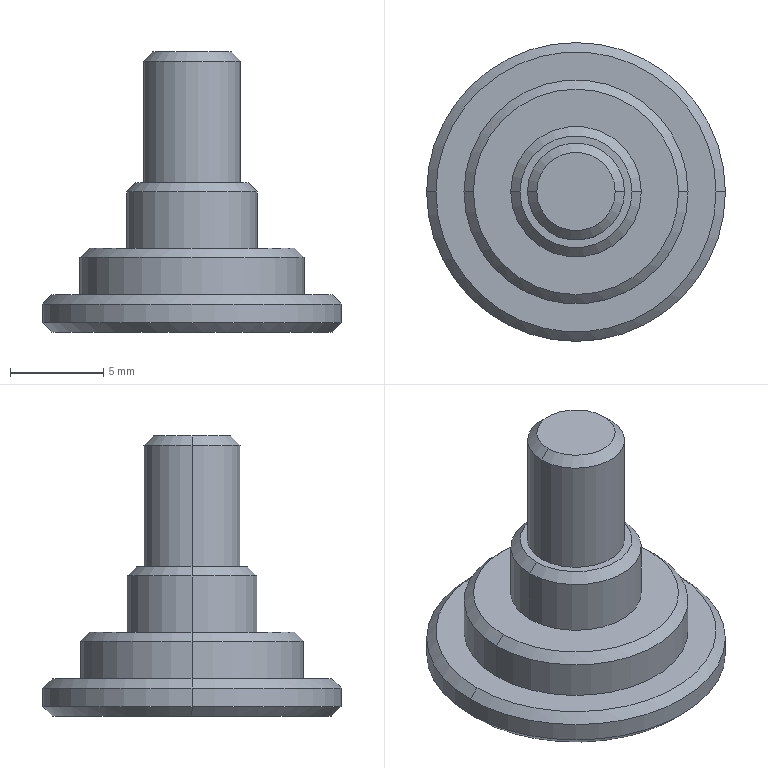Part | SolidWorks | features Boss 3, Chamfer 1, FlatPattern 1, SMBaseFlange 1, SheetMetal 1 | 1 solid | 23 faces | box 16 x 16 x 15 mm | volume 946.808 mm3 | cone 10 | cylinder 8 | plane 5 | commonest cylinder face diameters 5.2 x2 7 x2 12 x2 16 x2
STEP:
#1=CARTESIAN_POINT('',(2.1,0.,15.));
#2=VERTEX_POINT('',#1);
#3=CARTESIAN_POINT('',(-2.1,0.,15.));
#4=VERTEX_POINT('',#3);
#5=CARTESIAN_POINT('',(0.,0.,15.));
#6=DIRECTION('',(0.,0.,1.));
#7=DIRECTION('',(1.,0.,0.));
#8=AXIS2_PLACEMENT_3D('',#5,#6,#7);
#9=CIRCLE('',#8,2.1);
#10=EDGE_CURVE('',#2,#4,#9,.T.);
#11=ORIENTED_EDGE('',*,*,#10,.F.);
#12=CARTESIAN_POINT('',(2.6,0.,14.5));
#13=VERTEX_POINT('',#12);
#14=CARTESIAN_POINT('',(2.1,0.,15.));
#15=DIRECTION('',(0.7071,0.,-0.7071));
#16=VECTOR('',#15,1000.);
#17=LINE('',#14,#16);
#18=EDGE_CURVE('',#2,#13,#17,.T.);
#19=ORIENTED_EDGE('',*,*,#18,.T.);
#20=CARTESIAN_POINT('',(-2.6,0.,14.5));
#21=VERTEX_POINT('',#20);
#22=CARTESIAN_POINT('',(0.,0.,14.5));
#23=DIRECTION('',(0.,0.,-1.));
#24=DIRECTION('',(1.,0.,0.));
#25=AXIS2_PLACEMENT_3D('',#22,#23,#24);
#26=CIRCLE('',#25,2.6);
#27=EDGE_CURVE('',#21,#13,#26,.T.);
#28=ORIENTED_EDGE('',*,*,#27,.F.);
#29=CARTESIAN_POINT('',(-2.1,0.,15.));
#30=DIRECTION('',(-0.7071,0.,-0.7071));
#31=VECTOR('',#30,1000.);
#32=LINE('',#29,#31);
#33=EDGE_CURVE('',#4,#21,#32,.T.);
#34=ORIENTED_EDGE('',*,*,#33,.F.);
#35=EDGE_LOOP('',(#11,#19,#28,#34));
#36=FACE_OUTER_BOUND('',#35,.T.);
#37=CARTESIAN_POINT('',(0.,0.,15.));
#38=DIRECTION('',(0.,0.,-1.));
#39=DIRECTION('',(-1.,0.,0.));
#40=AXIS2_PLACEMENT_3D('',#37,#38,#39);
#41=CONICAL_SURFACE('',#40,2.1,0.7854);
#42=ADVANCED_FACE('',(#36),#41,.T.);
#43=CARTESIAN_POINT('',(3.,0.,8.));
#44=VERTEX_POINT('',#43);
#45=CARTESIAN_POINT('',(-3.,0.,8.));
#46=VERTEX_POINT('',#45);
#47=CARTESIAN_POINT('',(0.,0.,8.));
#48=DIRECTION('',(0.,0.,1.));
#49=DIRECTION('',(1.,0.,0.));
#50=AXIS2_PLACEMENT_3D('',#47,#48,#49);
#51=CIRCLE('',#50,3.);
#52=EDGE_CURVE('',#44,#46,#51,.T.);
#53=ORIENTED_EDGE('',*,*,#52,.F.);
#54=CARTESIAN_POINT('',(3.5,0.,7.5));
#55=VERTEX_POINT('',#54);
#56=CARTESIAN_POINT('',(3.,0.,8.));
#57=DIRECTION('',(0.7071,0.,-0.7071));
#58=VECTOR('',#57,1000.);
#59=LINE('',#56,#58);
#60=EDGE_CURVE('',#44,#55,#59,.T.);
#61=ORIENTED_EDGE('',*,*,#60,.T.);
#62=CARTESIAN_POINT('',(-3.5,0.,7.5));
#63=VERTEX_POINT('',#62);
#64=CARTESIAN_POINT('',(0.,0.,7.5));
#65=DIRECTION('',(0.,0.,-1.));
#66=DIRECTION('',(1.,0.,0.));
#67=AXIS2_PLACEMENT_3D('',#64,#65,#66);
#68=CIRCLE('',#67,3.5);
#69=EDGE_CURVE('',#63,#55,#68,.T.);
#70=ORIENTED_EDGE('',*,*,#69,.F.);
#71=CARTESIAN_POINT('',(-3.,0.,8.));
#72=DIRECTION('',(-0.7071,0.,-0.7071));
#73=VECTOR('',#72,1000.);
#74=LINE('',#71,#73);
#75=EDGE_CURVE('',#46,#63,#74,.T.);
#76=ORIENTED_EDGE('',*,*,#75,.F.);
#77=EDGE_LOOP('',(#53,#61,#70,#76));
#78=FACE_OUTER_BOUND('',#77,.T.);
#79=CARTESIAN_POINT('',(0.,0.,8.));
#80=DIRECTION('',(0.,0.,-1.));
#81=DIRECTION('',(-1.,0.,0.));
#82=AXIS2_PLACEMENT_3D('',#79,#80,#81);
#83=CONICAL_SURFACE('',#82,3.,0.7854);
#84=ADVANCED_FACE('',(#78),#83,.T.);
#85=CARTESIAN_POINT('',(5.5,0.,4.5));
#86=VERTEX_POINT('',#85);
#87=CARTESIAN_POINT('',(-5.5,0.,4.5));
#88=VERTEX_POINT('',#87);
#89=CARTESIAN_POINT('',(0.,0.,4.5));
#90=DIRECTION('',(0.,0.,1.));
#91=DIRECTION('',(1.,0.,0.));
#92=AXIS2_PLACEMENT_3D('',#89,#90,#91);
#93=CIRCLE('',#92,5.5);
#94=EDGE_CURVE('',#86,#88,#93,.T.);
#95=ORIENTED_EDGE('',*,*,#94,.F.);
#96=CARTESIAN_POINT('',(6.,0.,4.));
#97=VERTEX_POINT('',#96);
#98=CARTESIAN_POINT('',(5.5,0.,4.5));
#99=DIRECTION('',(0.7071,0.,-0.7071));
#100=VECTOR('',#99,1000.);
#101=LINE('',#98,#100);
#102=EDGE_CURVE('',#86,#97,#101,.T.);
#103=ORIENTED_EDGE('',*,*,#102,.T.);
#104=CARTESIAN_POINT('',(-6.,0.,4.));
#105=VERTEX_POINT('',#104);
#106=CARTESIAN_POINT('',(0.,0.,4.));
#107=DIRECTION('',(0.,0.,-1.));
#108=DIRECTION('',(1.,0.,0.));
#109=AXIS2_PLACEMENT_3D('',#106,#107,#108);
#110=CIRCLE('',#109,6.);
#111=EDGE_CURVE('',#105,#97,#110,.T.);
#112=ORIENTED_EDGE('',*,*,#111,.F.);
#113=CARTESIAN_POINT('',(-5.5,0.,4.5));
#114=DIRECTION('',(-0.7071,0.,-0.7071));
#115=VECTOR('',#114,1000.);
#116=LINE('',#113,#115);
#117=EDGE_CURVE('',#88,#105,#116,.T.);
#118=ORIENTED_EDGE('',*,*,#117,.F.);
#119=EDGE_LOOP('',(#95,#103,#112,#118));
#120=FACE_OUTER_BOUND('',#119,.T.);
#121=CARTESIAN_POINT('',(0.,0.,4.5));
#122=DIRECTION('',(0.,0.,-1.));
#123=DIRECTION('',(-1.,0.,0.));
#124=AXIS2_PLACEMENT_3D('',#121,#122,#123);
#125=CONICAL_SURFACE('',#124,5.5,0.7854);
#126=ADVANCED_FACE('',(#120),#125,.T.);
#127=CARTESIAN_POINT('',(7.5,0.,2.));
#128=VERTEX_POINT('',#127);
#129=CARTESIAN_POINT('',(-7.5,0.,2.));
#130=VERTEX_POINT('',#129);
#131=CARTESIAN_POINT('',(0.,0.,2.));
#132=DIRECTION('',(0.,0.,1.));
#133=DIRECTION('',(1.,0.,0.));
#134=AXIS2_PLACEMENT_3D('',#131,#132,#133);
#135=CIRCLE('',#134,7.5);
#136=EDGE_CURVE('',#128,#130,#135,.T.);
#137=ORIENTED_EDGE('',*,*,#136,.F.);
#138=CARTESIAN_POINT('',(8.,0.,1.5));
#139=VERTEX_POINT('',#138);
#140=CARTESIAN_POINT('',(7.5,0.,2.));
#141=DIRECTION('',(0.7071,0.,-0.7071));
#142=VECTOR('',#141,1000.);
#143=LINE('',#140,#142);
#144=EDGE_CURVE('',#128,#139,#143,.T.);
#145=ORIENTED_EDGE('',*,*,#144,.T.);
#146=CARTESIAN_POINT('',(-8.,0.,1.5));
#147=VERTEX_POINT('',#146);
#148=CARTESIAN_POINT('',(0.,0.,1.5));
#149=DIRECTION('',(0.,0.,-1.));
#150=DIRECTION('',(1.,0.,0.));
#151=AXIS2_PLACEMENT_3D('',#148,#149,#150);
#152=CIRCLE('',#151,8.);
#153=EDGE_CURVE('',#147,#139,#152,.T.);
#154=ORIENTED_EDGE('',*,*,#153,.F.);
#155=CARTESIAN_POINT('',(-7.5,0.,2.));
#156=DIRECTION('',(-0.7071,0.,-0.7071));
#157=VECTOR('',#156,1000.);
#158=LINE('',#155,#157);
#159=EDGE_CURVE('',#130,#147,#158,.T.);
#160=ORIENTED_EDGE('',*,*,#159,.F.);
#161=EDGE_LOOP('',(#137,#145,#154,#160));
#162=FACE_OUTER_BOUND('',#161,.T.);
#163=CARTESIAN_POINT('',(0.,0.,2.));
#164=DIRECTION('',(0.,0.,-1.));
#165=DIRECTION('',(-1.,0.,0.));
#166=AXIS2_PLACEMENT_3D('',#163,#164,#165);
#167=CONICAL_SURFACE('',#166,7.5,0.7854);
#168=ADVANCED_FACE('',(#162),#167,.T.);
#169=CARTESIAN_POINT('',(-7.5,0.,0.));
#170=VERTEX_POINT('',#169);
#171=CARTESIAN_POINT('',(7.5,0.,0.));
#172=VERTEX_POINT('',#171);
#173=CARTESIAN_POINT('',(0.,0.,0.));
#174=DIRECTION('',(0.,0.,-1.));
#175=DIRECTION('',(1.,0.,0.));
#176=AXIS2_PLACEMENT_3D('',#173,#174,#175);
#177=CIRCLE('',#176,7.5);
#178=EDGE_CURVE('',#170,#172,#177,.T.);
#179=ORIENTED_EDGE('',*,*,#178,.F.);
#180=CARTESIAN_POINT('',(-8.,0.,0.5));
#181=VERTEX_POINT('',#180);
#182=CARTESIAN_POINT('',(-8.,0.,0.5));
#183=DIRECTION('',(-0.7071,0.,0.7071));
#184=VECTOR('',#183,1000.);
#185=LINE('',#182,#184);
#186=EDGE_CURVE('',#170,#181,#185,.T.);
#187=ORIENTED_EDGE('',*,*,#186,.T.);
#188=CARTESIAN_POINT('',(8.,0.,0.5));
#189=VERTEX_POINT('',#188);
#190=CARTESIAN_POINT('',(0.,0.,0.5));
#191=DIRECTION('',(0.,0.,1.));
#192=DIRECTION('',(1.,0.,0.));
#193=AXIS2_PLACEMENT_3D('',#190,#191,#192);
#194=CIRCLE('',#193,8.);
#195=EDGE_CURVE('',#189,#181,#194,.T.);
#196=ORIENTED_EDGE('',*,*,#195,.F.);
#197=CARTESIAN_POINT('',(8.,0.,0.5));
#198=DIRECTION('',(0.7071,0.,0.7071));
#199=VECTOR('',#198,1000.);
#200=LINE('',#197,#199);
#201=EDGE_CURVE('',#172,#189,#200,.T.);
#202=ORIENTED_EDGE('',*,*,#201,.F.);
#203=EDGE_LOOP('',(#179,#187,#196,#202));
#204=FACE_OUTER_BOUND('',#203,.T.);
#205=CARTESIAN_POINT('',(0.,0.,0.5));
#206=DIRECTION('',(0.,0.,1.));
#207=DIRECTION('',(1.,0.,0.));
#208=AXIS2_PLACEMENT_3D('',#205,#206,#207);
#209=CONICAL_SURFACE('',#208,8.,0.7854);
#210=ADVANCED_FACE('',(#204),#209,.T.);
#211=ORIENTED_EDGE('',*,*,#27,.T.);
#212=CARTESIAN_POINT('',(2.6,0.,8.));
#213=VERTEX_POINT('',#212);
#214=CARTESIAN_POINT('',(2.6,0.,15.));
#215=DIRECTION('',(0.,0.,-1.));
#216=VECTOR('',#215,1000.);
#217=LINE('',#214,#216);
#218=EDGE_CURVE('',#13,#213,#217,.T.);
#219=ORIENTED_EDGE('',*,*,#218,.T.);
#220=CARTESIAN_POINT('',(-2.6,0.,8.));
#221=VERTEX_POINT('',#220);
#222=CARTESIAN_POINT('',(0.,0.,8.));
#223=DIRECTION('',(0.,0.,1.));
#224=DIRECTION('',(1.,0.,0.));
#225=AXIS2_PLACEMENT_3D('',#222,#223,#224);
#226=CIRCLE('',#225,2.6);
#227=EDGE_CURVE('',#213,#221,#226,.T.);
#228=ORIENTED_EDGE('',*,*,#227,.T.);
#229=CARTESIAN_POINT('',(-2.6,0.,15.));
#230=DIRECTION('',(0.,0.,-1.));
#231=VECTOR('',#230,1000.);
#232=LINE('',#229,#231);
#233=EDGE_CURVE('',#21,#221,#232,.T.);
#234=ORIENTED_EDGE('',*,*,#233,.F.);
#235=EDGE_LOOP('',(#211,#219,#228,#234));
#236=FACE_OUTER_BOUND('',#235,.T.);
#237=CARTESIAN_POINT('',(0.,0.,15.));
#238=DIRECTION('',(0.,0.,-1.));
#239=DIRECTION('',(-1.,0.,0.));
#240=AXIS2_PLACEMENT_3D('',#237,#238,#239);
#241=CYLINDRICAL_SURFACE('',#240,2.6);
#242=ADVANCED_FACE('',(#236),#241,.T.);
#243=ORIENTED_EDGE('',*,*,#69,.T.);
#244=CARTESIAN_POINT('',(3.5,0.,4.5));
#245=VERTEX_POINT('',#244);
#246=CARTESIAN_POINT('',(3.5,0.,8.));
#247=DIRECTION('',(0.,0.,-1.));
#248=VECTOR('',#247,1000.);
#249=LINE('',#246,#248);
#250=EDGE_CURVE('',#55,#245,#249,.T.);
#251=ORIENTED_EDGE('',*,*,#250,.T.);
#252=CARTESIAN_POINT('',(-3.5,0.,4.5));
#253=VERTEX_POINT('',#252);
#254=CARTESIAN_POINT('',(0.,0.,4.5));
#255=DIRECTION('',(0.,0.,1.));
#256=DIRECTION('',(1.,0.,0.));
#257=AXIS2_PLACEMENT_3D('',#254,#255,#256);
#258=CIRCLE('',#257,3.5);
#259=EDGE_CURVE('',#245,#253,#258,.T.);
#260=ORIENTED_EDGE('',*,*,#259,.T.);
#261=CARTESIAN_POINT('',(-3.5,0.,8.));
#262=DIRECTION('',(0.,0.,-1.));
#263=VECTOR('',#262,1000.);
#264=LINE('',#261,#263);
#265=EDGE_CURVE('',#63,#253,#264,.T.);
#266=ORIENTED_EDGE('',*,*,#265,.F.);
#267=EDGE_LOOP('',(#243,#251,#260,#266));
#268=FACE_OUTER_BOUND('',#267,.T.);
#269=CARTESIAN_POINT('',(0.,0.,8.));
#270=DIRECTION('',(0.,0.,-1.));
#271=DIRECTION('',(-1.,0.,0.));
#272=AXIS2_PLACEMENT_3D('',#269,#270,#271);
#273=CYLINDRICAL_SURFACE('',#272,3.5);
#274=ADVANCED_FACE('',(#268),#273,.T.);
#275=ORIENTED_EDGE('',*,*,#111,.T.);
#276=CARTESIAN_POINT('',(6.,0.,2.));
#277=VERTEX_POINT('',#276);
#278=CARTESIAN_POINT('',(6.,0.,4.5));
#279=DIRECTION('',(0.,0.,-1.));
#280=VECTOR('',#279,1000.);
#281=LINE('',#278,#280);
#282=EDGE_CURVE('',#97,#277,#281,.T.);
#283=ORIENTED_EDGE('',*,*,#282,.T.);
#284=CARTESIAN_POINT('',(-6.,0.,2.));
#285=VERTEX_POINT('',#284);
#286=CARTESIAN_POINT('',(0.,0.,2.));
#287=DIRECTION('',(0.,0.,1.));
#288=DIRECTION('',(1.,0.,0.));
#289=AXIS2_PLACEMENT_3D('',#286,#287,#288);
#290=CIRCLE('',#289,6.);
#291=EDGE_CURVE('',#277,#285,#290,.T.);
#292=ORIENTED_EDGE('',*,*,#291,.T.);
#293=CARTESIAN_POINT('',(-6.,0.,4.5));
#294=DIRECTION('',(0.,0.,-1.));
#295=VECTOR('',#294,1000.);
#296=LINE('',#293,#295);
#297=EDGE_CURVE('',#105,#285,#296,.T.);
#298=ORIENTED_EDGE('',*,*,#297,.F.);
#299=EDGE_LOOP('',(#275,#283,#292,#298));
#300=FACE_OUTER_BOUND('',#299,.T.);
#301=CARTESIAN_POINT('',(0.,0.,4.5));
#302=DIRECTION('',(0.,0.,-1.));
#303=DIRECTION('',(-1.,0.,0.));
#304=AXIS2_PLACEMENT_3D('',#301,#302,#303);
#305=CYLINDRICAL_SURFACE('',#304,6.);
#306=ADVANCED_FACE('',(#300),#305,.T.);
#307=ORIENTED_EDGE('',*,*,#153,.T.);
#308=CARTESIAN_POINT('',(8.,0.,2.));
#309=DIRECTION('',(0.,0.,-1.));
#310=VECTOR('',#309,1000.);
#311=LINE('',#308,#310);
#312=EDGE_CURVE('',#139,#189,#311,.T.);
#313=ORIENTED_EDGE('',*,*,#312,.T.);
#314=ORIENTED_EDGE('',*,*,#195,.T.);
#315=CARTESIAN_POINT('',(-8.,0.,2.));
#316=DIRECTION('',(0.,0.,-1.));
#317=VECTOR('',#316,1000.);
#318=LINE('',#315,#317);
#319=EDGE_CURVE('',#147,#181,#318,.T.);
#320=ORIENTED_EDGE('',*,*,#319,.F.);
#321=EDGE_LOOP('',(#307,#313,#314,#320));
#322=FACE_OUTER_BOUND('',#321,.T.);
#323=CARTESIAN_POINT('',(0.,0.,2.));
#324=DIRECTION('',(0.,0.,-1.));
#325=DIRECTION('',(-1.,0.,0.));
#326=AXIS2_PLACEMENT_3D('',#323,#324,#325);
#327=CYLINDRICAL_SURFACE('',#326,8.);
#328=ADVANCED_FACE('',(#322),#327,.T.);
#329=CARTESIAN_POINT('',(0.,0.,8.));
#330=DIRECTION('',(0.,0.,1.));
#331=DIRECTION('',(1.,0.,0.));
#332=AXIS2_PLACEMENT_3D('',#329,#330,#331);
#333=CIRCLE('',#332,3.);
#334=EDGE_CURVE('',#46,#44,#333,.T.);
#335=ORIENTED_EDGE('',*,*,#334,.T.);
#336=ORIENTED_EDGE('',*,*,#52,.T.);
#337=EDGE_LOOP('',(#335,#336));
#338=FACE_OUTER_BOUND('',#337,.T.);
#339=CARTESIAN_POINT('',(0.,0.,8.));
#340=DIRECTION('',(0.,0.,1.));
#341=DIRECTION('',(1.,0.,0.));
#342=AXIS2_PLACEMENT_3D('',#339,#340,#341);
#343=CIRCLE('',#342,2.6);
#344=EDGE_CURVE('',#221,#213,#343,.T.);
#345=ORIENTED_EDGE('',*,*,#344,.F.);
#346=ORIENTED_EDGE('',*,*,#227,.F.);
#347=EDGE_LOOP('',(#345,#346));
#348=FACE_BOUND('',#347,.T.);
#349=CARTESIAN_POINT('',(0.,0.,8.));
#350=DIRECTION('',(0.,0.,1.));
#351=DIRECTION('',(1.,0.,0.));
#352=AXIS2_PLACEMENT_3D('',#349,#350,#351);
#353=PLANE('',#352);
#354=ADVANCED_FACE('',(#338,#348),#353,.T.);
#355=CARTESIAN_POINT('',(0.,0.,4.5));
#356=DIRECTION('',(0.,0.,1.));
#357=DIRECTION('',(1.,0.,0.));
#358=AXIS2_PLACEMENT_3D('',#355,#356,#357);
#359=CIRCLE('',#358,5.5);
#360=EDGE_CURVE('',#88,#86,#359,.T.);
#361=ORIENTED_EDGE('',*,*,#360,.T.);
#362=ORIENTED_EDGE('',*,*,#94,.T.);
#363=EDGE_LOOP('',(#361,#362));
#364=FACE_OUTER_BOUND('',#363,.T.);
#365=CARTESIAN_POINT('',(0.,0.,4.5));
#366=DIRECTION('',(0.,0.,1.));
#367=DIRECTION('',(1.,0.,0.));
#368=AXIS2_PLACEMENT_3D('',#365,#366,#367);
#369=CIRCLE('',#368,3.5);
#370=EDGE_CURVE('',#253,#245,#369,.T.);
#371=ORIENTED_EDGE('',*,*,#370,.F.);
#372=ORIENTED_EDGE('',*,*,#259,.F.);
#373=EDGE_LOOP('',(#371,#372));
#374=FACE_BOUND('',#373,.T.);
#375=CARTESIAN_POINT('',(0.,0.,4.5));
#376=DIRECTION('',(0.,0.,1.));
#377=DIRECTION('',(1.,0.,0.));
#378=AXIS2_PLACEMENT_3D('',#375,#376,#377);
#379=PLANE('',#378);
#380=ADVANCED_FACE('',(#364,#374),#379,.T.);
#381=CARTESIAN_POINT('',(0.,0.,2.));
#382=DIRECTION('',(0.,0.,1.));
#383=DIRECTION('',(1.,0.,0.));
#384=AXIS2_PLACEMENT_3D('',#381,#382,#383);
#385=CIRCLE('',#384,7.5);
#386=EDGE_CURVE('',#130,#128,#385,.T.);
#387=ORIENTED_EDGE('',*,*,#386,.T.);
#388=ORIENTED_EDGE('',*,*,#136,.T.);
#389=EDGE_LOOP('',(#387,#388));
#390=FACE_OUTER_BOUND('',#389,.T.);
#391=CARTESIAN_POINT('',(0.,0.,2.));
#392=DIRECTION('',(0.,0.,1.));
#393=DIRECTION('',(1.,0.,0.));
#394=AXIS2_PLACEMENT_3D('',#391,#392,#393);
#395=CIRCLE('',#394,6.);
#396=EDGE_CURVE('',#285,#277,#395,.T.);
#397=ORIENTED_EDGE('',*,*,#396,.F.);
#398=ORIENTED_EDGE('',*,*,#291,.F.);
#399=EDGE_LOOP('',(#397,#398));
#400=FACE_BOUND('',#399,.T.);
#401=CARTESIAN_POINT('',(0.,0.,2.));
#402=DIRECTION('',(0.,0.,1.));
#403=DIRECTION('',(1.,0.,0.));
#404=AXIS2_PLACEMENT_3D('',#401,#402,#403);
#405=PLANE('',#404);
#406=ADVANCED_FACE('',(#390,#400),#405,.T.);
#407=ORIENTED_EDGE('',*,*,#312,.F.);
#408=CARTESIAN_POINT('',(0.,0.,1.5));
#409=DIRECTION('',(0.,0.,-1.));
#410=DIRECTION('',(1.,0.,0.));
#411=AXIS2_PLACEMENT_3D('',#408,#409,#410);
#412=CIRCLE('',#411,8.);
#413=EDGE_CURVE('',#139,#147,#412,.T.);
#414=ORIENTED_EDGE('',*,*,#413,.T.);
#415=ORIENTED_EDGE('',*,*,#319,.T.);
#416=CARTESIAN_POINT('',(0.,0.,0.5));
#417=DIRECTION('',(0.,0.,1.));
#418=DIRECTION('',(1.,0.,0.));
#419=AXIS2_PLACEMENT_3D('',#416,#417,#418);
#420=CIRCLE('',#419,8.);
#421=EDGE_CURVE('',#181,#189,#420,.T.);
#422=ORIENTED_EDGE('',*,*,#421,.T.);
#423=EDGE_LOOP('',(#407,#414,#415,#422));
#424=FACE_OUTER_BOUND('',#423,.T.);
#425=CARTESIAN_POINT('',(0.,0.,2.));
#426=DIRECTION('',(0.,0.,-1.));
#427=DIRECTION('',(-1.,0.,0.));
#428=AXIS2_PLACEMENT_3D('',#425,#426,#427);
#429=CYLINDRICAL_SURFACE('',#428,8.);
#430=ADVANCED_FACE('',(#424),#429,.T.);
#431=CARTESIAN_POINT('',(0.,0.,0.));
#432=DIRECTION('',(0.,0.,-1.));
#433=DIRECTION('',(1.,0.,0.));
#434=AXIS2_PLACEMENT_3D('',#431,#432,#433);
#435=CIRCLE('',#434,7.5);
#436=EDGE_CURVE('',#172,#170,#435,.T.);
#437=ORIENTED_EDGE('',*,*,#436,.T.);
#438=ORIENTED_EDGE('',*,*,#178,.T.);
#439=EDGE_LOOP('',(#437,#438));
#440=FACE_OUTER_BOUND('',#439,.T.);
#441=CARTESIAN_POINT('',(0.,0.,0.));
#442=DIRECTION('',(0.,0.,1.));
#443=DIRECTION('',(1.,0.,0.));
#444=AXIS2_PLACEMENT_3D('',#441,#442,#443);
#445=PLANE('',#444);
#446=ADVANCED_FACE('',(#440),#445,.F.);
#447=ORIENTED_EDGE('',*,*,#282,.F.);
#448=CARTESIAN_POINT('',(0.,0.,4.));
#449=DIRECTION('',(0.,0.,-1.));
#450=DIRECTION('',(1.,0.,0.));
#451=AXIS2_PLACEMENT_3D('',#448,#449,#450);
#452=CIRCLE('',#451,6.);
#453=EDGE_CURVE('',#97,#105,#452,.T.);
#454=ORIENTED_EDGE('',*,*,#453,.T.);
#455=ORIENTED_EDGE('',*,*,#297,.T.);
#456=ORIENTED_EDGE('',*,*,#396,.T.);
#457=EDGE_LOOP('',(#447,#454,#455,#456));
#458=FACE_OUTER_BOUND('',#457,.T.);
#459=CARTESIAN_POINT('',(0.,0.,4.5));
#460=DIRECTION('',(0.,0.,-1.));
#461=DIRECTION('',(-1.,0.,0.));
#462=AXIS2_PLACEMENT_3D('',#459,#460,#461);
#463=CYLINDRICAL_SURFACE('',#462,6.);
#464=ADVANCED_FACE('',(#458),#463,.T.);
#465=ORIENTED_EDGE('',*,*,#250,.F.);
#466=CARTESIAN_POINT('',(0.,0.,7.5));
#467=DIRECTION('',(0.,0.,-1.));
#468=DIRECTION('',(1.,0.,0.));
#469=AXIS2_PLACEMENT_3D('',#466,#467,#468);
#470=CIRCLE('',#469,3.5);
#471=EDGE_CURVE('',#55,#63,#470,.T.);
#472=ORIENTED_EDGE('',*,*,#471,.T.);
#473=ORIENTED_EDGE('',*,*,#265,.T.);
#474=ORIENTED_EDGE('',*,*,#370,.T.);
#475=EDGE_LOOP('',(#465,#472,#473,#474));
#476=FACE_OUTER_BOUND('',#475,.T.);
#477=CARTESIAN_POINT('',(0.,0.,8.));
#478=DIRECTION('',(0.,0.,-1.));
#479=DIRECTION('',(-1.,0.,0.));
#480=AXIS2_PLACEMENT_3D('',#477,#478,#479);
#481=CYLINDRICAL_SURFACE('',#480,3.5);
#482=ADVANCED_FACE('',(#476),#481,.T.);
#483=ORIENTED_EDGE('',*,*,#218,.F.);
#484=CARTESIAN_POINT('',(0.,0.,14.5));
#485=DIRECTION('',(0.,0.,-1.));
#486=DIRECTION('',(1.,0.,0.));
#487=AXIS2_PLACEMENT_3D('',#484,#485,#486);
#488=CIRCLE('',#487,2.6);
#489=EDGE_CURVE('',#13,#21,#488,.T.);
#490=ORIENTED_EDGE('',*,*,#489,.T.);
#491=ORIENTED_EDGE('',*,*,#233,.T.);
#492=ORIENTED_EDGE('',*,*,#344,.T.);
#493=EDGE_LOOP('',(#483,#490,#491,#492));
#494=FACE_OUTER_BOUND('',#493,.T.);
#495=CARTESIAN_POINT('',(0.,0.,15.));
#496=DIRECTION('',(0.,0.,-1.));
#497=DIRECTION('',(-1.,0.,0.));
#498=AXIS2_PLACEMENT_3D('',#495,#496,#497);
#499=CYLINDRICAL_SURFACE('',#498,2.6);
#500=ADVANCED_FACE('',(#494),#499,.T.);
#501=CARTESIAN_POINT('',(0.,0.,15.));
#502=DIRECTION('',(0.,0.,1.));
#503=DIRECTION('',(1.,0.,0.));
#504=AXIS2_PLACEMENT_3D('',#501,#502,#503);
#505=CIRCLE('',#504,2.1);
#506=EDGE_CURVE('',#4,#2,#505,.T.);
#507=ORIENTED_EDGE('',*,*,#506,.T.);
#508=ORIENTED_EDGE('',*,*,#10,.T.);
#509=EDGE_LOOP('',(#507,#508));
#510=FACE_OUTER_BOUND('',#509,.T.);
#511=CARTESIAN_POINT('',(0.,0.,15.));
#512=DIRECTION('',(0.,0.,1.));
#513=DIRECTION('',(1.,0.,0.));
#514=AXIS2_PLACEMENT_3D('',#511,#512,#513);
#515=PLANE('',#514);
#516=ADVANCED_FACE('',(#510),#515,.T.);
#517=ORIENTED_EDGE('',*,*,#186,.F.);
#518=ORIENTED_EDGE('',*,*,#436,.F.);
#519=ORIENTED_EDGE('',*,*,#201,.T.);
#520=ORIENTED_EDGE('',*,*,#421,.F.);
#521=EDGE_LOOP('',(#517,#518,#519,#520));
#522=FACE_OUTER_BOUND('',#521,.T.);
#523=CARTESIAN_POINT('',(0.,0.,0.5));
#524=DIRECTION('',(0.,0.,1.));
#525=DIRECTION('',(1.,0.,0.));
#526=AXIS2_PLACEMENT_3D('',#523,#524,#525);
#527=CONICAL_SURFACE('',#526,8.,0.7854);
#528=ADVANCED_FACE('',(#522),#527,.T.);
#529=ORIENTED_EDGE('',*,*,#144,.F.);
#530=ORIENTED_EDGE('',*,*,#386,.F.);
#531=ORIENTED_EDGE('',*,*,#159,.T.);
#532=ORIENTED_EDGE('',*,*,#413,.F.);
#533=EDGE_LOOP('',(#529,#530,#531,#532));
#534=FACE_OUTER_BOUND('',#533,.T.);
#535=CARTESIAN_POINT('',(0.,0.,2.));
#536=DIRECTION('',(0.,0.,-1.));
#537=DIRECTION('',(-1.,0.,0.));
#538=AXIS2_PLACEMENT_3D('',#535,#536,#537);
#539=CONICAL_SURFACE('',#538,7.5,0.7854);
#540=ADVANCED_FACE('',(#534),#539,.T.);
#541=ORIENTED_EDGE('',*,*,#102,.F.);
#542=ORIENTED_EDGE('',*,*,#360,.F.);
#543=ORIENTED_EDGE('',*,*,#117,.T.);
#544=ORIENTED_EDGE('',*,*,#453,.F.);
#545=EDGE_LOOP('',(#541,#542,#543,#544));
#546=FACE_OUTER_BOUND('',#545,.T.);
#547=CARTESIAN_POINT('',(0.,0.,4.5));
#548=DIRECTION('',(0.,0.,-1.));
#549=DIRECTION('',(-1.,0.,0.));
#550=AXIS2_PLACEMENT_3D('',#547,#548,#549);
#551=CONICAL_SURFACE('',#550,5.5,0.7854);
#552=ADVANCED_FACE('',(#546),#551,.T.);
#553=ORIENTED_EDGE('',*,*,#60,.F.);
#554=ORIENTED_EDGE('',*,*,#334,.F.);
#555=ORIENTED_EDGE('',*,*,#75,.T.);
#556=ORIENTED_EDGE('',*,*,#471,.F.);
#557=EDGE_LOOP('',(#553,#554,#555,#556));
#558=FACE_OUTER_BOUND('',#557,.T.);
#559=CARTESIAN_POINT('',(0.,0.,8.));
#560=DIRECTION('',(0.,0.,-1.));
#561=DIRECTION('',(-1.,0.,0.));
#562=AXIS2_PLACEMENT_3D('',#559,#560,#561);
#563=CONICAL_SURFACE('',#562,3.,0.7854);
#564=ADVANCED_FACE('',(#558),#563,.T.);
#565=ORIENTED_EDGE('',*,*,#18,.F.);
#566=ORIENTED_EDGE('',*,*,#506,.F.);
#567=ORIENTED_EDGE('',*,*,#33,.T.);
#568=ORIENTED_EDGE('',*,*,#489,.F.);
#569=EDGE_LOOP('',(#565,#566,#567,#568));
#570=FACE_OUTER_BOUND('',#569,.T.);
#571=CARTESIAN_POINT('',(0.,0.,15.));
#572=DIRECTION('',(0.,0.,-1.));
#573=DIRECTION('',(-1.,0.,0.));
#574=AXIS2_PLACEMENT_3D('',#571,#572,#573);
#575=CONICAL_SURFACE('',#574,2.1,0.7854);
#576=ADVANCED_FACE('',(#570),#575,.T.);
#577=CLOSED_SHELL('',(#42,#84,#126,#168,#210,#242,#274,#306,#328,#354,#380,#406,#430,#446,#464,#482,#500,#516,#528,#540,#552,#564,#576));
#578=MANIFOLD_SOLID_BREP('',#577);
#579=CARTESIAN_POINT('',(0.,0.,0.));
#580=DIRECTION('',(0.,0.,1.));
#581=DIRECTION('',(1.,0.,0.));
#582=AXIS2_PLACEMENT_3D('',#579,#580,#581);
#583=(LENGTH_UNIT()NAMED_UNIT(*)SI_UNIT(.MILLI.,.METRE.));
#584=UNCERTAINTY_MEASURE_WITH_UNIT(LENGTH_MEASURE(0.00001),#583,'','');
#585=(NAMED_UNIT(*)PLANE_ANGLE_UNIT()SI_UNIT($,.RADIAN.));
#586=(NAMED_UNIT(*)SI_UNIT($,.STERADIAN.)SOLID_ANGLE_UNIT());
#587=(GEOMETRIC_REPRESENTATION_CONTEXT(3)GLOBAL_UNCERTAINTY_ASSIGNED_CONTEXT((#584))GLOBAL_UNIT_ASSIGNED_CONTEXT((#583,#585,#586))REPRESENTATION_CONTEXT('',''));
#588=ADVANCED_BREP_SHAPE_REPRESENTATION('',(#578,#582),#587);